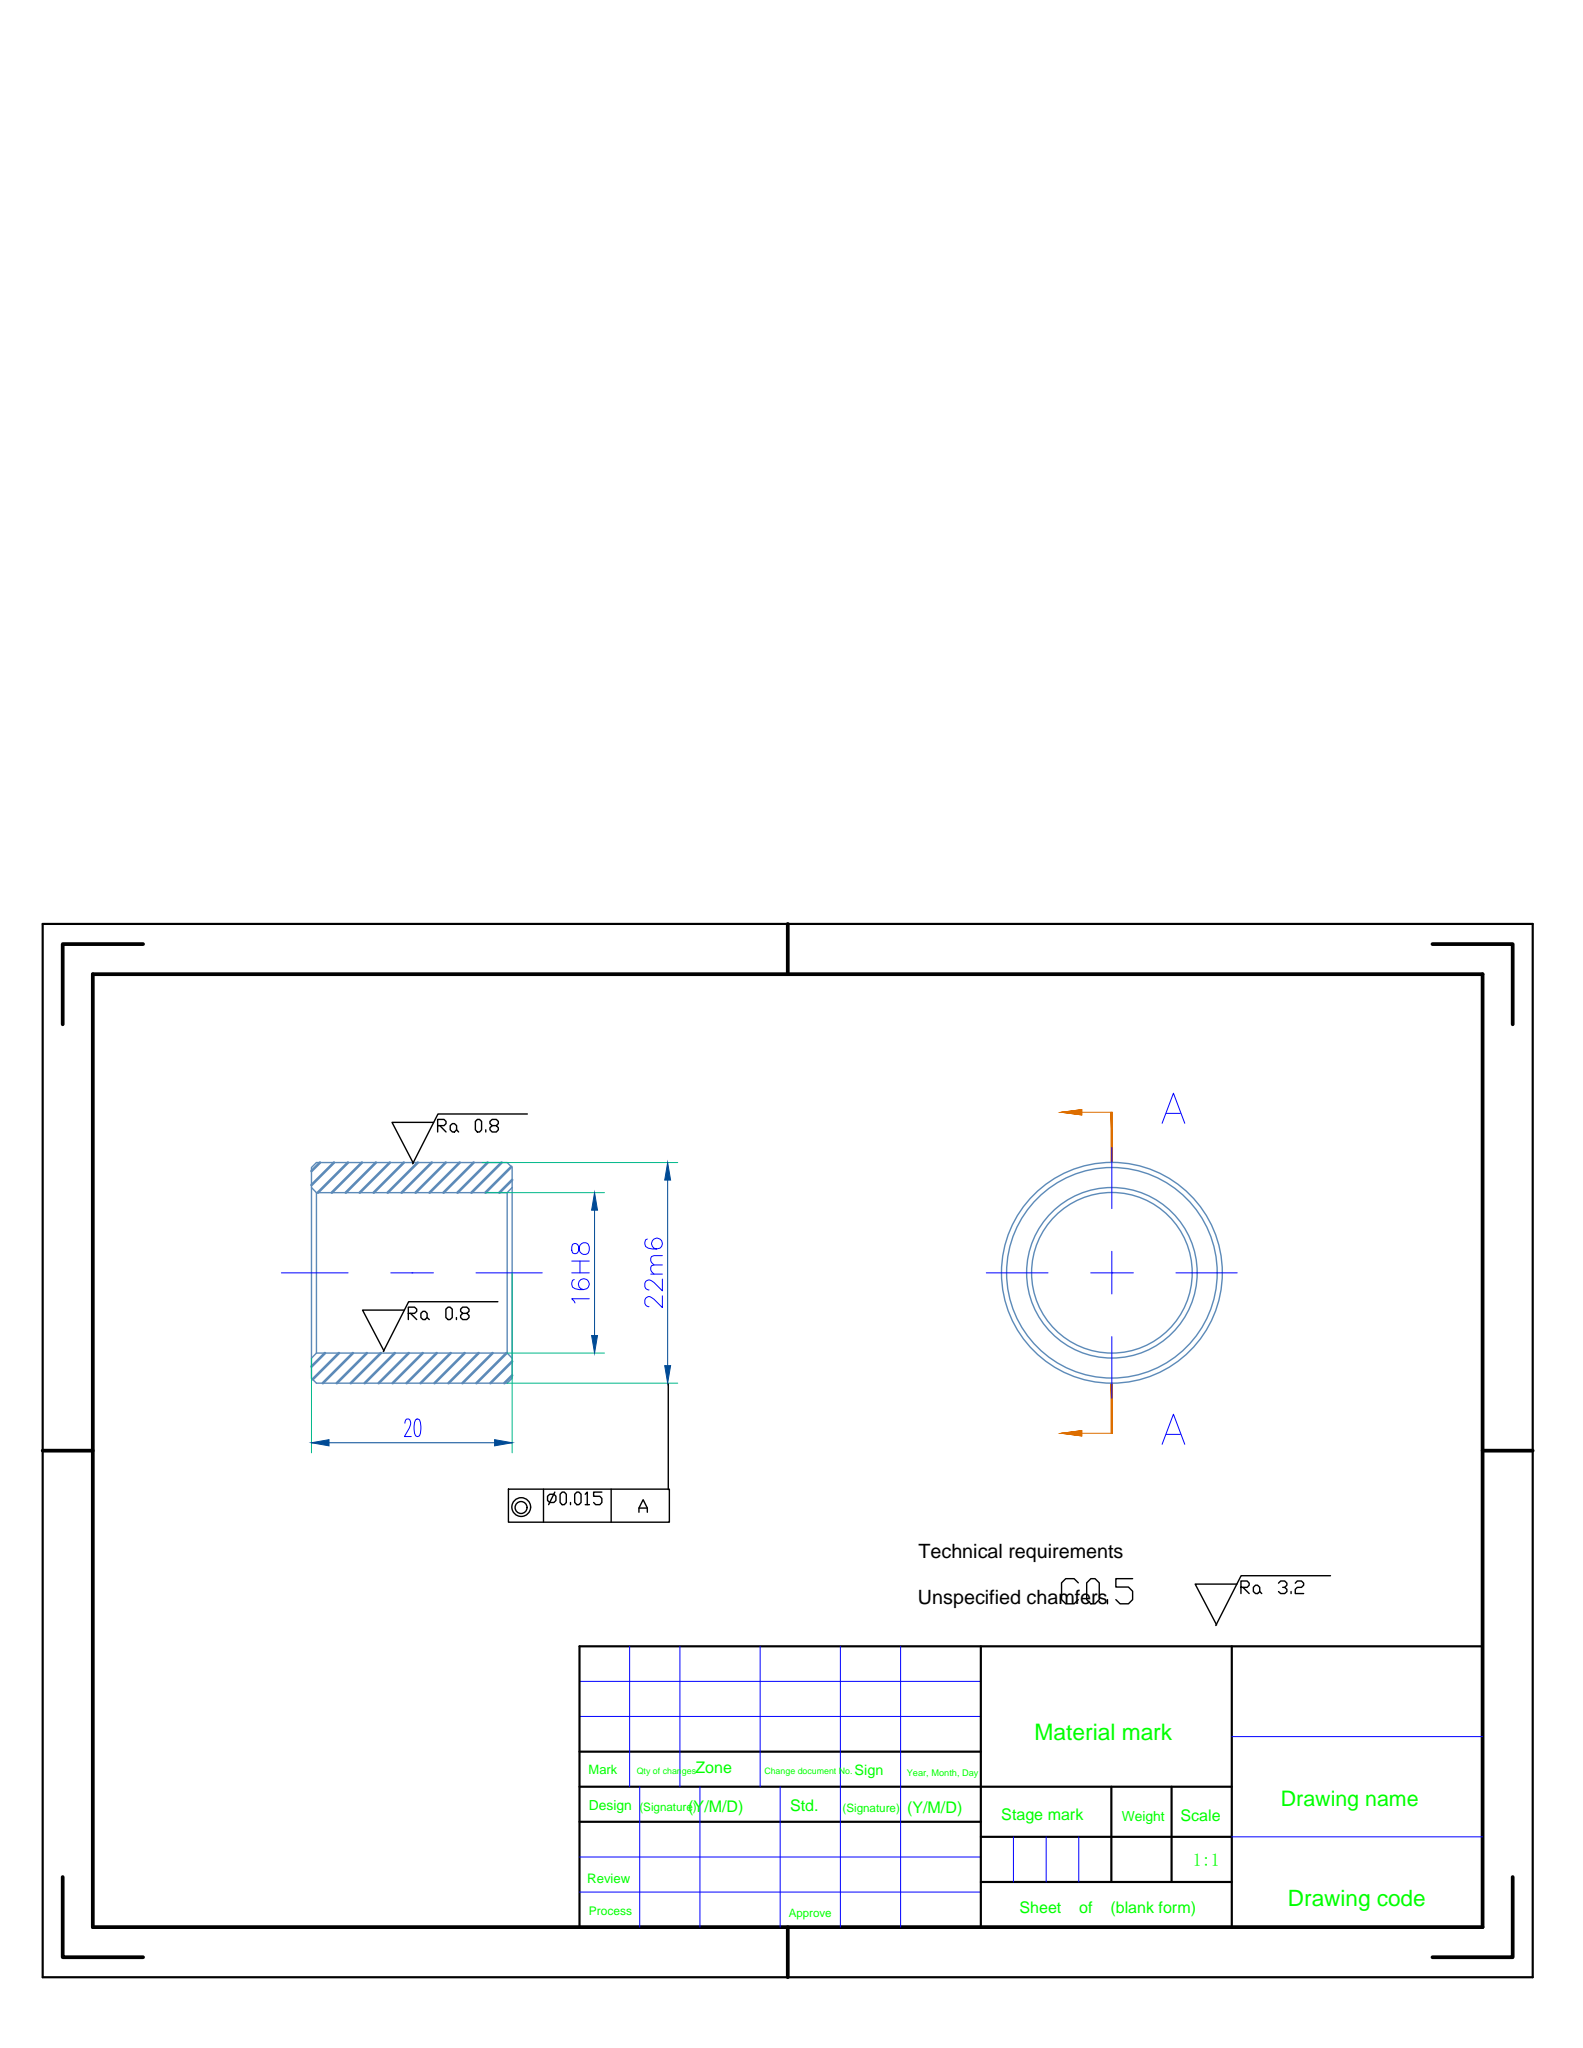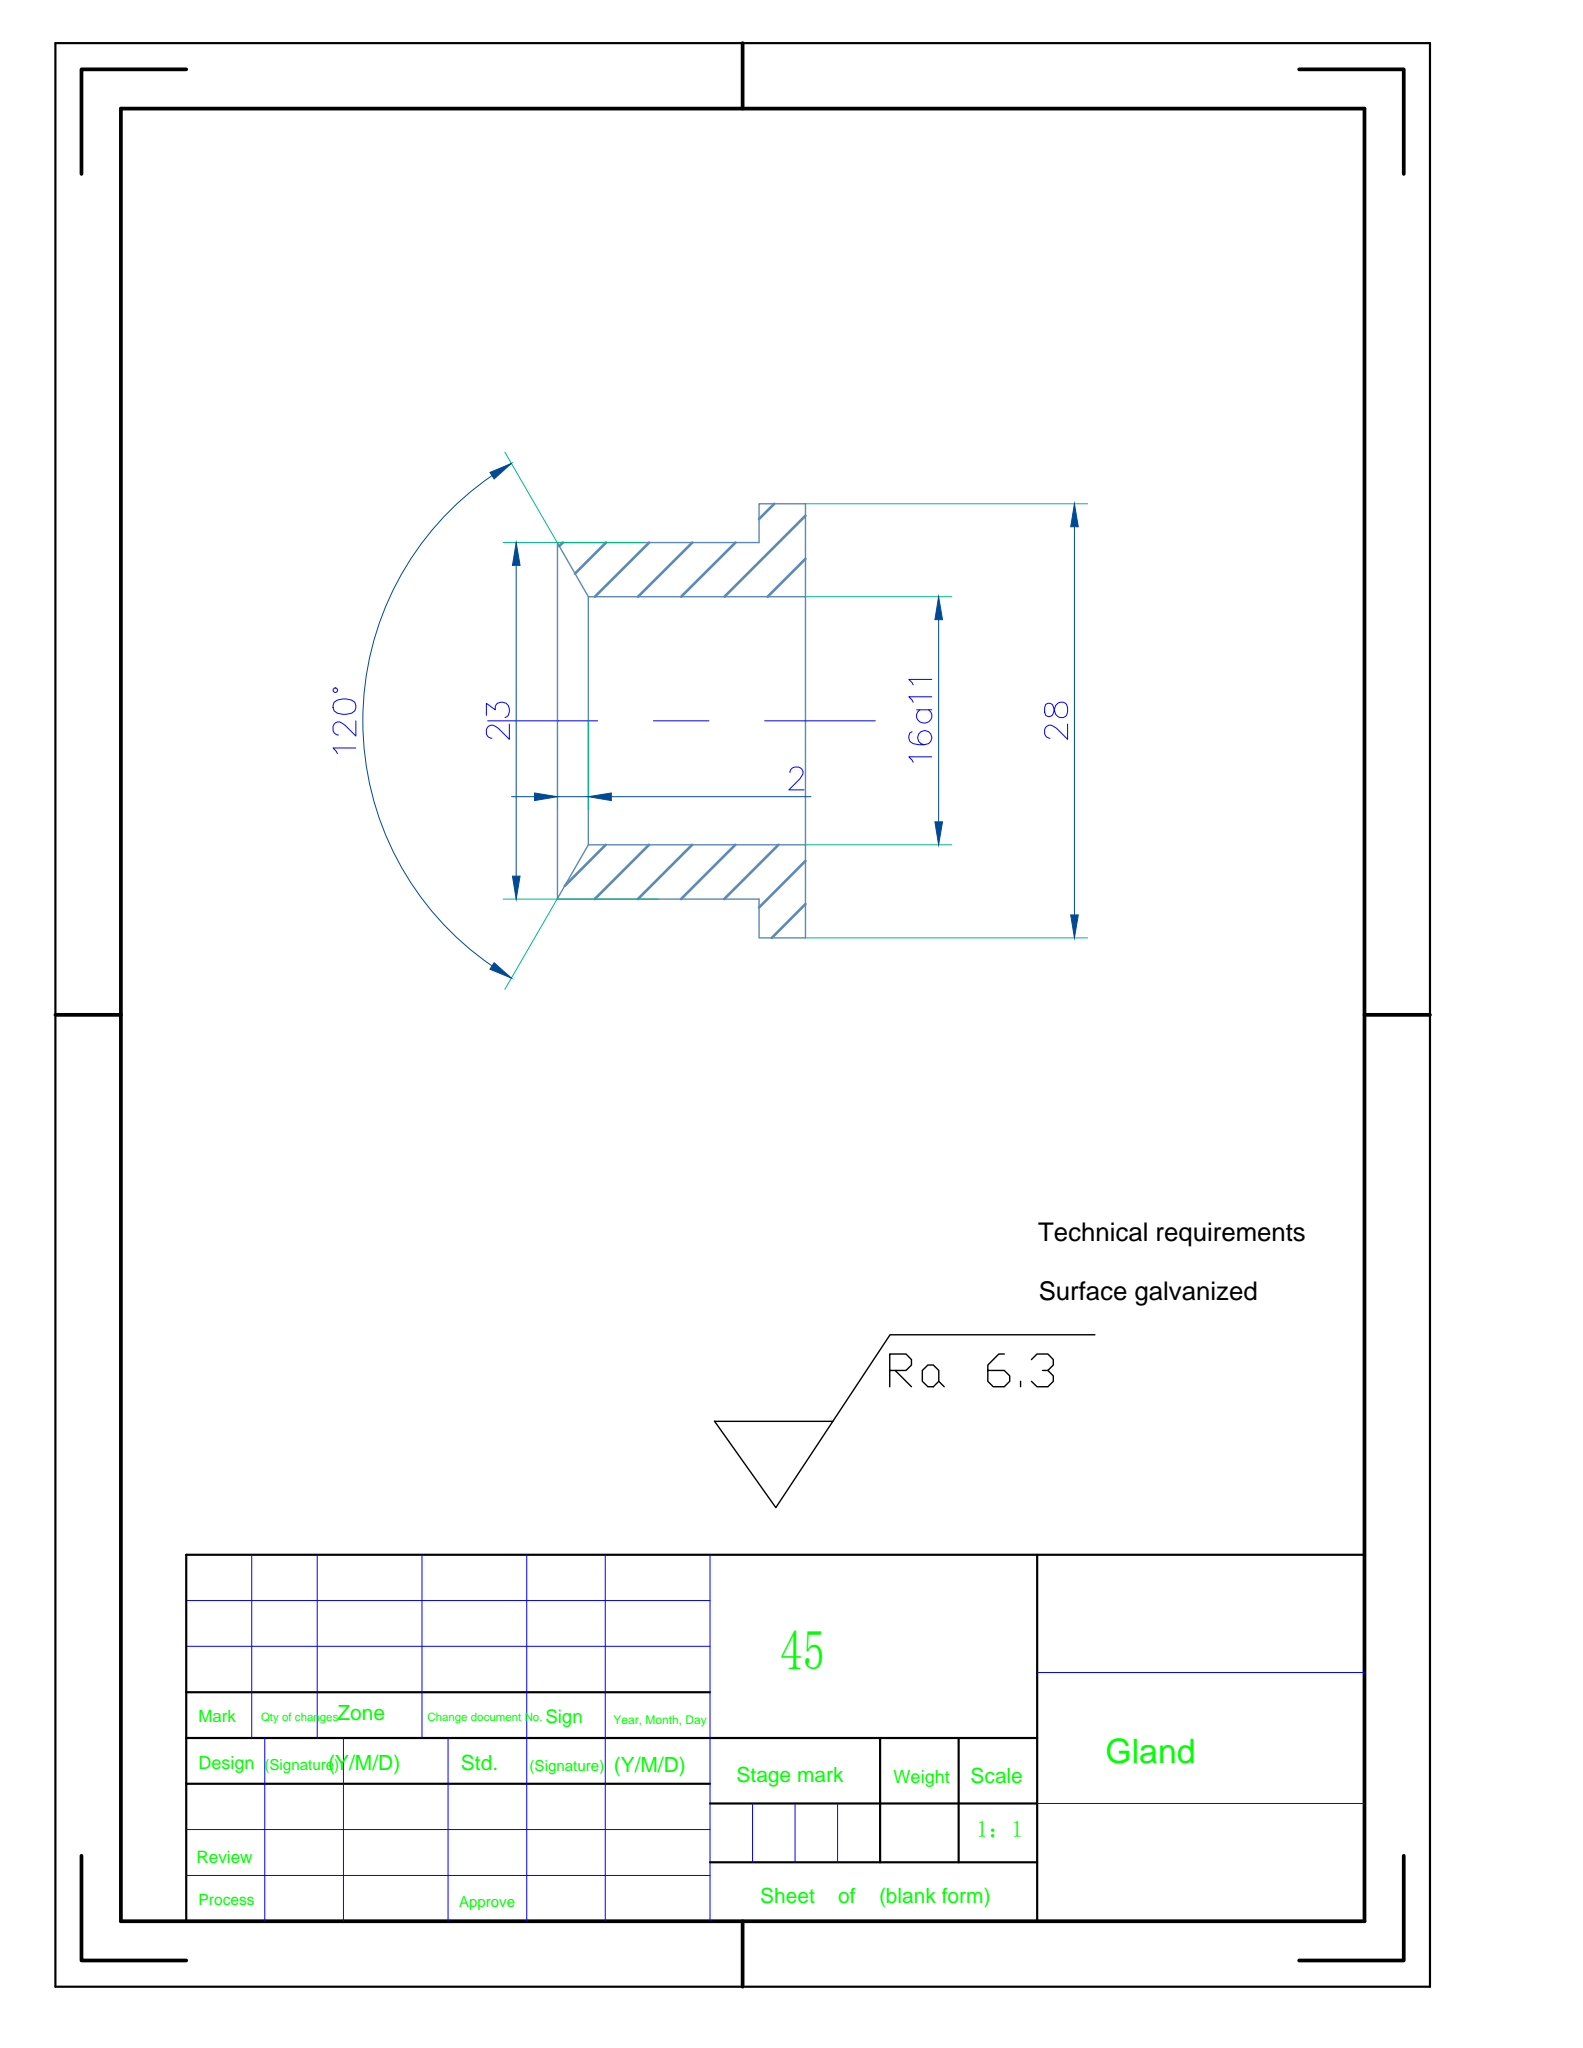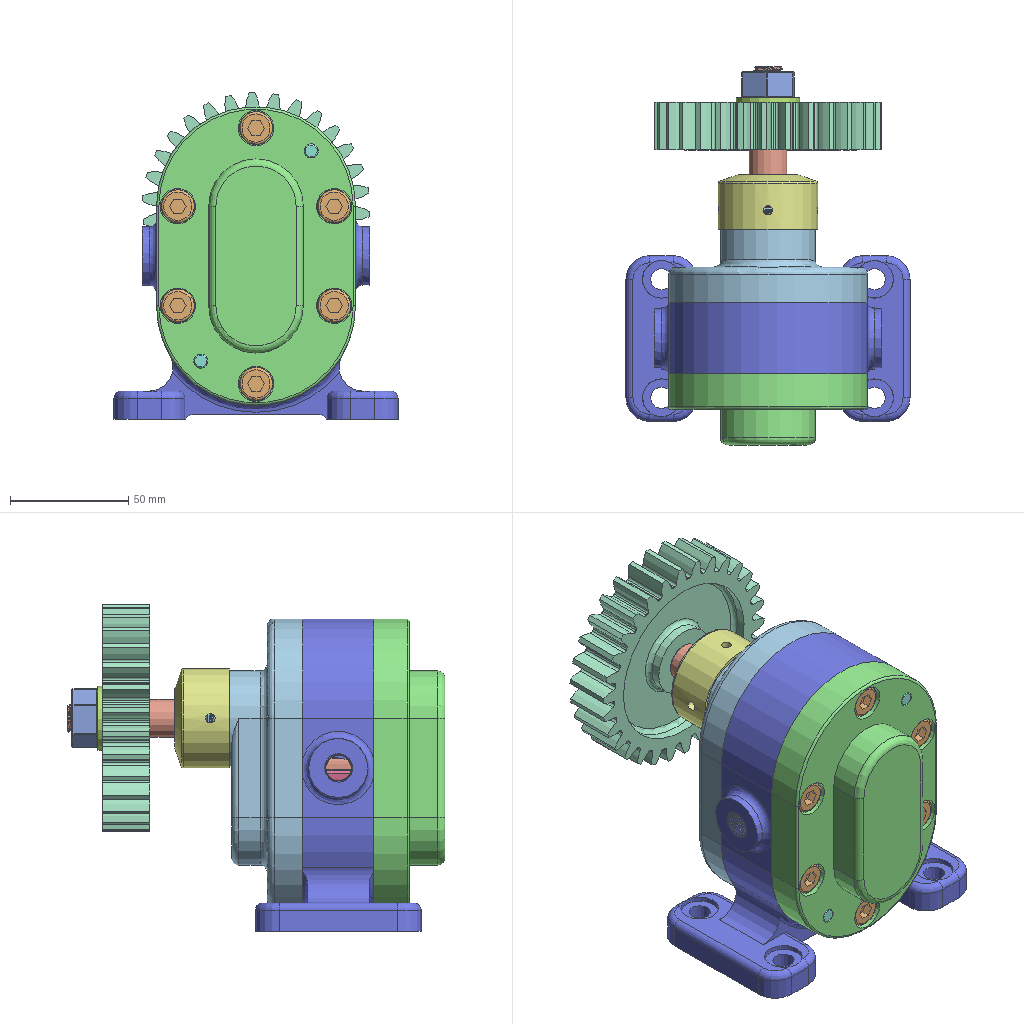Assembly | NX | 15 different items | 33 placed | box 120 x 160 x 138 mm
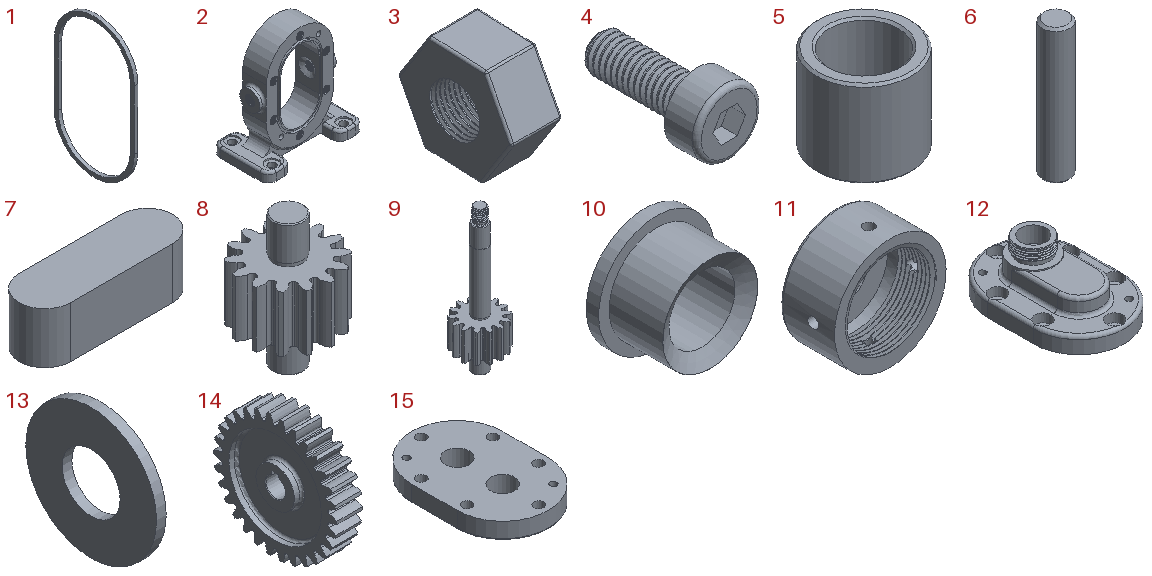Parts list (item | quantity | size | volume | features):
1 | x2 | 2.5 x 56.6 x 98.6 mm | 1771 mm3 | features DATUM_CSYS 2, DATUM_PLANE 1, EXTRUDE 1, SKETCH 1
2 | x1 | 120 x 70 x 132 mm | 199459 mm3 | features EXTRUDE 12, THREADS 8, DATUM_CSYS 7, DATUM_PLANE 6, EXTRACT_STRING 6, SKETCH 6, BLEND 5, CHAMFER 4, EXTRACT_FACE 4, Instance Feature 2, Mirror Feature 2
3 | x1 | 11 x 24.824 x 22.141 mm | 3308 mm3 | features BLEND 2, DATUM_CSYS 2, DATUM_PLANE 1, EXTRUDE 1, SKETCH 1, THREADS 1
4 | x12 | 14 x 28 x 14 mm | 1799 mm3 | features DATUM_CSYS 3, EXTRUDE 3, DATUM_PLANE 2, SKETCH 2, BLEND 1, CHAMFER 1, THREADS 1
5 | x4 | 22 x 22 x 20 mm | 3552 mm3 | features DATUM_CSYS 2, CHAMFER 1, DATUM_PLANE 1, EXTRUDE 1, SKETCH 1
6 | x4 | 6 x 6 x 30 mm | 843.779 mm3 | features CHAMFER 1, CYLINDER 1, DATUM_CSYS 1
7 | x1 | 15 x 5 x 5 mm | 348.175 mm3 | features DATUM_CSYS 2, DATUM_PLANE 1, EXTRUDE 1, SKETCH 1
8 | x1 | 47.19 x 48 x 70 mm | 48349 mm3 | features BREP 14, META 14, CYLINDER 3, CHAMFER 2, DATUM_CSYS 2, EXTRACT_FACE 2, EXTRACT_STRING 2, EXTRUDE 2, DATUM_PLANE 1, FSET 1, Instance Feature 1, Mirror Feature 1, SKETCH 1
9 | x1 | 47.19 x 48 x 150 mm | 62108 mm3 | features BREP 14, META 14, CYLINDER 5, DATUM_CSYS 5, DATUM_PLANE 4, EXTRUDE 4, SKETCH 4, CHAMFER 3, BLEND 1, FSET 1, THREADS 1
10 | x1 | 28 x 16 x 28 mm | 3832 mm3 | features DATUM_CSYS 2, DATUM_PLANE 1, SKETCH 1, SWP104 1
11 | x1 | 42 x 23 x 42 mm | 14105 mm3 | features DATUM_CSYS 5, SKETCH 4, EXTRUDE 3, BLEND 1, SWP104 1, THREADS 1
12 | x1 | 84 x 126 x 45 mm | 154692 mm3 | features DATUM_CSYS 7, EXTRUDE 7, DATUM_PLANE 6, SKETCH 6, EXTRACT_STRING 2, SWP104 2, BLEND 1, CHAMFER 1, HOLE PACKAGE 1, Instance Feature 1, Mirror Feature 1, SIMPLE HOLE 1, THREADS 1
13 | x1 | 2 x 27 x 27 mm | 918.916 mm3 | features DATUM_CSYS 2, DATUM_PLANE 1, EXTRUDE 1, SKETCH 1
14 | x1 | 20 x 96 x 95.68 mm | 82292 mm3 | features BREP 30, META 30, EXTRUDE 3, DATUM_CSYS 2, EXTRACT_FACE 2, EXTRACT_STRING 2, BLEND 1, CHAMFER 1, CYLINDER 1, DATUM_PLANE 1, FSET 1, Instance Feature 1, Mirror Feature 1, SKETCH 1
15 | x1 | 84 x 126 x 30 mm | 151500 mm3 | features CBORE_HOLE 6, DATUM_CSYS 6, SKETCH 5, SIMPLE HOLE 4, EXTRUDE 3, HOLE PACKAGE 3, BLEND 2
Mates (type | each side: item.copy, entity, surface, feature):
Fix | 2.1 component
Concentric | 15.1 edge | 2.1 edge | 2 times
Concentric | 9.1 edge | 15.1 edge
Concentric | 8.1 edge | 15.1 edge
Concentric | 12.1 edge | 2.1 edge
Concentric | 5.1 edge | 15.1 edge | 2 times
Concentric | 5.1 edge | 12.1 edge | 2 times
Concentric | 10.1 edge | 12.1 edge
Concentric | 11.1 edge | 10.1 edge
Concentric | 14.1 edge | 9.1 edge
Concentric | 4.1 edge | 15.1 edge | 6 times
Concentric | 4.1 edge | 12.1 edge | 6 times
Concentric | 6.1 edge | 15.1 edge | 2 times
Concentric | 6.1 edge | 12.1 edge | 2 times
Concentric | 1.1 edge | 2.1 edge | 2 times
Concentric | 13.1 edge | 14.1 edge
Concentric | 3.1 edge | 13.1 edge
Concentric | 7.1 edge | 9.1 edge
Parallel | 7.1 edge | 9.1 edge